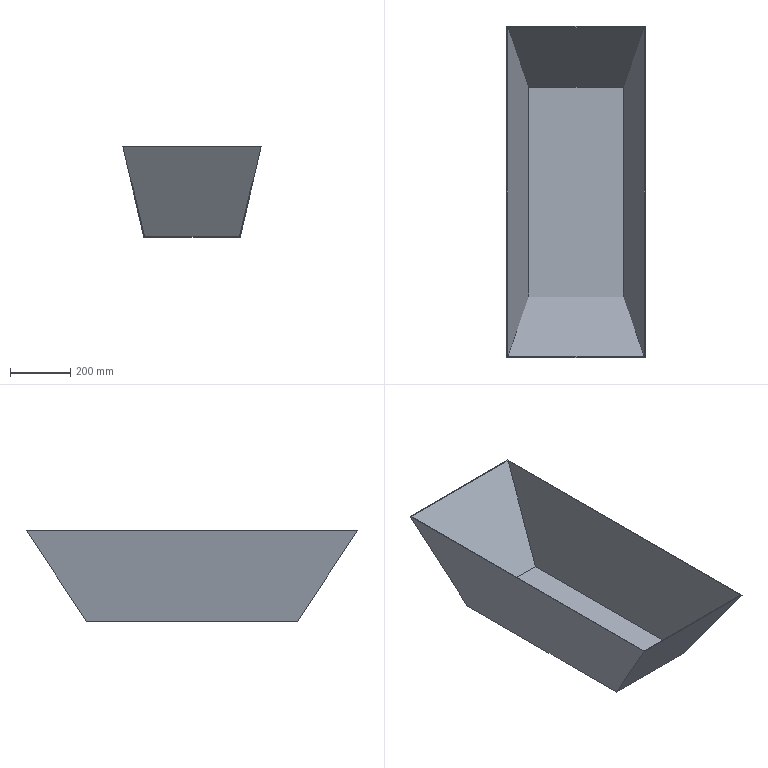Part | SolidWorks | features ICE 2, Extrusion 1, Shell 1 | 1 solid | 11 faces | box 460 x 1100 x 300 mm | volume 3149502 mm3 | plane 11
STEP:
#1=CARTESIAN_POINT('',(-160.,350.,-300.));
#2=VERTEX_POINT('',#1);
#3=CARTESIAN_POINT('',(160.,350.,-300.));
#4=VERTEX_POINT('',#3);
#5=CARTESIAN_POINT('',(-230.,350.,-300.));
#6=DIRECTION('',(1.,0.,0.));
#7=VECTOR('',#6,1000.);
#8=LINE('',#5,#7);
#9=EDGE_CURVE('',#2,#4,#8,.T.);
#10=ORIENTED_EDGE('',*,*,#9,.T.);
#11=CARTESIAN_POINT('',(160.,-350.,-300.));
#12=VERTEX_POINT('',#11);
#13=CARTESIAN_POINT('',(160.,-949.,-300.));
#14=DIRECTION('',(0.,1.,0.));
#15=VECTOR('',#14,1000.);
#16=LINE('',#13,#15);
#17=EDGE_CURVE('',#12,#4,#16,.T.);
#18=ORIENTED_EDGE('',*,*,#17,.F.);
#19=CARTESIAN_POINT('',(-160.,-350.,-300.));
#20=VERTEX_POINT('',#19);
#21=CARTESIAN_POINT('',(-230.,-350.,-300.));
#22=DIRECTION('',(1.,0.,0.));
#23=VECTOR('',#22,1000.);
#24=LINE('',#21,#23);
#25=EDGE_CURVE('',#20,#12,#24,.T.);
#26=ORIENTED_EDGE('',*,*,#25,.F.);
#27=CARTESIAN_POINT('',(-160.,-949.,-300.));
#28=DIRECTION('',(0.,1.,0.));
#29=VECTOR('',#28,1000.);
#30=LINE('',#27,#29);
#31=EDGE_CURVE('',#20,#2,#30,.T.);
#32=ORIENTED_EDGE('',*,*,#31,.T.);
#33=EDGE_LOOP('',(#10,#18,#26,#32));
#34=FACE_OUTER_BOUND('',#33,.T.);
#35=CARTESIAN_POINT('',(0.,0.,-300.));
#36=DIRECTION('',(0.,0.,1.));
#37=DIRECTION('',(1.,0.,0.));
#38=AXIS2_PLACEMENT_3D('',#35,#36,#37);
#39=PLANE('',#38);
#40=ADVANCED_FACE('',(#34),#39,.F.);
#41=CARTESIAN_POINT('',(226.919,-546.394,0.));
#42=VERTEX_POINT('',#41);
#43=CARTESIAN_POINT('',(226.919,546.394,0.));
#44=VERTEX_POINT('',#43);
#45=CARTESIAN_POINT('',(226.919,-949.,0.));
#46=DIRECTION('',(0.,1.,0.));
#47=VECTOR('',#46,1000.);
#48=LINE('',#45,#47);
#49=EDGE_CURVE('',#42,#44,#48,.T.);
#50=ORIENTED_EDGE('',*,*,#49,.F.);
#51=CARTESIAN_POINT('',(-226.919,-546.394,0.));
#52=VERTEX_POINT('',#51);
#53=CARTESIAN_POINT('',(-230.,-546.394,0.));
#54=DIRECTION('',(1.,0.,0.));
#55=VECTOR('',#54,1000.);
#56=LINE('',#53,#55);
#57=EDGE_CURVE('',#52,#42,#56,.T.);
#58=ORIENTED_EDGE('',*,*,#57,.F.);
#59=CARTESIAN_POINT('',(-226.919,546.394,0.));
#60=VERTEX_POINT('',#59);
#61=CARTESIAN_POINT('',(-226.919,-949.,0.));
#62=DIRECTION('',(0.,-1.,0.));
#63=VECTOR('',#62,1000.);
#64=LINE('',#61,#63);
#65=EDGE_CURVE('',#60,#52,#64,.T.);
#66=ORIENTED_EDGE('',*,*,#65,.F.);
#67=CARTESIAN_POINT('',(-230.,546.394,0.));
#68=DIRECTION('',(-1.,0.,0.));
#69=VECTOR('',#68,1000.);
#70=LINE('',#67,#69);
#71=EDGE_CURVE('',#44,#60,#70,.T.);
#72=ORIENTED_EDGE('',*,*,#71,.F.);
#73=EDGE_LOOP('',(#50,#58,#66,#72));
#74=FACE_BOUND('',#73,.T.);
#75=CARTESIAN_POINT('',(230.,-550.,0.));
#76=VERTEX_POINT('',#75);
#77=CARTESIAN_POINT('',(230.,550.,0.));
#78=VERTEX_POINT('',#77);
#79=CARTESIAN_POINT('',(230.,550.,0.));
#80=DIRECTION('',(0.,1.,0.));
#81=VECTOR('',#80,1000.);
#82=LINE('',#79,#81);
#83=EDGE_CURVE('',#76,#78,#82,.T.);
#84=ORIENTED_EDGE('',*,*,#83,.T.);
#85=CARTESIAN_POINT('',(-230.,550.,0.));
#86=VERTEX_POINT('',#85);
#87=CARTESIAN_POINT('',(-230.,550.,0.));
#88=DIRECTION('',(-1.,0.,0.));
#89=VECTOR('',#88,1000.);
#90=LINE('',#87,#89);
#91=EDGE_CURVE('',#78,#86,#90,.T.);
#92=ORIENTED_EDGE('',*,*,#91,.T.);
#93=CARTESIAN_POINT('',(-230.,-550.,0.));
#94=VERTEX_POINT('',#93);
#95=CARTESIAN_POINT('',(-230.,550.,0.));
#96=DIRECTION('',(0.,-1.,0.));
#97=VECTOR('',#96,1000.);
#98=LINE('',#95,#97);
#99=EDGE_CURVE('',#86,#94,#98,.T.);
#100=ORIENTED_EDGE('',*,*,#99,.T.);
#101=CARTESIAN_POINT('',(-230.,-550.,0.));
#102=DIRECTION('',(1.,0.,0.));
#103=VECTOR('',#102,1000.);
#104=LINE('',#101,#103);
#105=EDGE_CURVE('',#94,#76,#104,.T.);
#106=ORIENTED_EDGE('',*,*,#105,.T.);
#107=EDGE_LOOP('',(#84,#92,#100,#106));
#108=FACE_OUTER_BOUND('',#107,.T.);
#109=CARTESIAN_POINT('',(0.,0.,0.));
#110=DIRECTION('',(0.,0.,1.));
#111=DIRECTION('',(1.,0.,0.));
#112=AXIS2_PLACEMENT_3D('',#109,#110,#111);
#113=PLANE('',#112);
#114=ADVANCED_FACE('',(#74,#108),#113,.T.);
#115=ORIENTED_EDGE('',*,*,#91,.F.);
#116=CARTESIAN_POINT('',(213.291,502.261,-71.609));
#117=DIRECTION('',(-0.1906,-0.5445,-0.8168));
#118=VECTOR('',#117,1000.);
#119=LINE('',#116,#118);
#120=EDGE_CURVE('',#78,#4,#119,.T.);
#121=ORIENTED_EDGE('',*,*,#120,.T.);
#122=ORIENTED_EDGE('',*,*,#9,.F.);
#123=CARTESIAN_POINT('',(-230.,550.,0.));
#124=DIRECTION('',(-0.1906,0.5445,0.8168));
#125=VECTOR('',#124,1000.);
#126=LINE('',#123,#125);
#127=EDGE_CURVE('',#2,#86,#126,.T.);
#128=ORIENTED_EDGE('',*,*,#127,.T.);
#129=EDGE_LOOP('',(#115,#121,#122,#128));
#130=FACE_OUTER_BOUND('',#129,.T.);
#131=CARTESIAN_POINT('',(-230.,550.,0.));
#132=DIRECTION('',(0.,-0.8321,0.5547));
#133=DIRECTION('',(0.,-0.5547,-0.8321));
#134=AXIS2_PLACEMENT_3D('',#131,#132,#133);
#135=PLANE('',#134);
#136=ADVANCED_FACE('',(#130),#135,.F.);
#137=ORIENTED_EDGE('',*,*,#25,.T.);
#138=CARTESIAN_POINT('',(213.291,-502.261,-71.609));
#139=DIRECTION('',(0.1906,-0.5445,0.8168));
#140=VECTOR('',#139,1000.);
#141=LINE('',#138,#140);
#142=EDGE_CURVE('',#12,#76,#141,.T.);
#143=ORIENTED_EDGE('',*,*,#142,.T.);
#144=ORIENTED_EDGE('',*,*,#105,.F.);
#145=CARTESIAN_POINT('',(-230.,-550.,0.));
#146=DIRECTION('',(0.1906,0.5445,-0.8168));
#147=VECTOR('',#146,1000.);
#148=LINE('',#145,#147);
#149=EDGE_CURVE('',#94,#20,#148,.T.);
#150=ORIENTED_EDGE('',*,*,#149,.T.);
#151=EDGE_LOOP('',(#137,#143,#144,#150));
#152=FACE_OUTER_BOUND('',#151,.T.);
#153=CARTESIAN_POINT('',(-230.,-550.,0.));
#154=DIRECTION('',(0.,0.8321,0.5547));
#155=DIRECTION('',(0.,-0.5547,0.8321));
#156=AXIS2_PLACEMENT_3D('',#153,#154,#155);
#157=PLANE('',#156);
#158=ADVANCED_FACE('',(#152),#157,.F.);
#159=ORIENTED_EDGE('',*,*,#31,.F.);
#160=ORIENTED_EDGE('',*,*,#149,.F.);
#161=ORIENTED_EDGE('',*,*,#99,.F.);
#162=ORIENTED_EDGE('',*,*,#127,.F.);
#163=EDGE_LOOP('',(#159,#160,#161,#162));
#164=FACE_OUTER_BOUND('',#163,.T.);
#165=CARTESIAN_POINT('',(-230.,-949.,0.));
#166=DIRECTION('',(0.9738,0.,0.2272));
#167=DIRECTION('',(0.2272,0.,-0.9738));
#168=AXIS2_PLACEMENT_3D('',#165,#166,#167);
#169=PLANE('',#168);
#170=ADVANCED_FACE('',(#164),#169,.F.);
#171=ORIENTED_EDGE('',*,*,#83,.F.);
#172=ORIENTED_EDGE('',*,*,#142,.F.);
#173=ORIENTED_EDGE('',*,*,#17,.T.);
#174=ORIENTED_EDGE('',*,*,#120,.F.);
#175=EDGE_LOOP('',(#171,#172,#173,#174));
#176=FACE_OUTER_BOUND('',#175,.T.);
#177=CARTESIAN_POINT('',(230.,-949.,0.));
#178=DIRECTION('',(-0.9738,0.,0.2272));
#179=DIRECTION('',(0.2272,0.,0.9738));
#180=AXIS2_PLACEMENT_3D('',#177,#178,#179);
#181=PLANE('',#180);
#182=ADVANCED_FACE('',(#176),#181,.F.);
#183=CARTESIAN_POINT('',(-157.619,348.394,-297.));
#184=VERTEX_POINT('',#183);
#185=CARTESIAN_POINT('',(157.619,348.394,-297.));
#186=VERTEX_POINT('',#185);
#187=CARTESIAN_POINT('',(0.,348.394,-297.));
#188=DIRECTION('',(1.,0.,0.));
#189=VECTOR('',#188,1000.);
#190=LINE('',#187,#189);
#191=EDGE_CURVE('',#184,#186,#190,.T.);
#192=ORIENTED_EDGE('',*,*,#191,.F.);
#193=CARTESIAN_POINT('',(-157.619,-348.394,-297.));
#194=VERTEX_POINT('',#193);
#195=CARTESIAN_POINT('',(-157.619,0.,-297.));
#196=DIRECTION('',(0.,1.,0.));
#197=VECTOR('',#196,1000.);
#198=LINE('',#195,#197);
#199=EDGE_CURVE('',#194,#184,#198,.T.);
#200=ORIENTED_EDGE('',*,*,#199,.F.);
#201=CARTESIAN_POINT('',(157.619,-348.394,-297.));
#202=VERTEX_POINT('',#201);
#203=CARTESIAN_POINT('',(-230.,-348.394,-297.));
#204=DIRECTION('',(1.,0.,0.));
#205=VECTOR('',#204,1000.);
#206=LINE('',#203,#205);
#207=EDGE_CURVE('',#194,#202,#206,.T.);
#208=ORIENTED_EDGE('',*,*,#207,.T.);
#209=CARTESIAN_POINT('',(157.619,-949.,-297.));
#210=DIRECTION('',(0.,1.,0.));
#211=VECTOR('',#210,1000.);
#212=LINE('',#209,#211);
#213=EDGE_CURVE('',#202,#186,#212,.T.);
#214=ORIENTED_EDGE('',*,*,#213,.T.);
#215=EDGE_LOOP('',(#192,#200,#208,#214));
#216=FACE_OUTER_BOUND('',#215,.T.);
#217=CARTESIAN_POINT('',(0.,0.,-297.));
#218=DIRECTION('',(0.,0.,1.));
#219=DIRECTION('',(1.,0.,0.));
#220=AXIS2_PLACEMENT_3D('',#217,#218,#219);
#221=PLANE('',#220);
#222=ADVANCED_FACE('',(#216),#221,.T.);
#223=ORIENTED_EDGE('',*,*,#71,.T.);
#224=CARTESIAN_POINT('',(-227.405,547.783,2.083));
#225=DIRECTION('',(-0.1906,0.5445,0.8168));
#226=VECTOR('',#225,1000.);
#227=LINE('',#224,#226);
#228=EDGE_CURVE('',#184,#60,#227,.T.);
#229=ORIENTED_EDGE('',*,*,#228,.F.);
#230=ORIENTED_EDGE('',*,*,#191,.T.);
#231=CARTESIAN_POINT('',(210.697,500.044,-69.525));
#232=DIRECTION('',(-0.1906,-0.5445,-0.8168));
#233=VECTOR('',#232,1000.);
#234=LINE('',#231,#233);
#235=EDGE_CURVE('',#44,#186,#234,.T.);
#236=ORIENTED_EDGE('',*,*,#235,.F.);
#237=EDGE_LOOP('',(#223,#229,#230,#236));
#238=FACE_OUTER_BOUND('',#237,.T.);
#239=CARTESIAN_POINT('',(-230.,547.504,1.664));
#240=DIRECTION('',(0.,-0.8321,0.5547));
#241=DIRECTION('',(0.,-0.5547,-0.8321));
#242=AXIS2_PLACEMENT_3D('',#239,#240,#241);
#243=PLANE('',#242);
#244=ADVANCED_FACE('',(#238),#243,.T.);
#245=ORIENTED_EDGE('',*,*,#207,.F.);
#246=CARTESIAN_POINT('',(-227.405,-547.783,2.083));
#247=DIRECTION('',(0.1906,0.5445,-0.8168));
#248=VECTOR('',#247,1000.);
#249=LINE('',#246,#248);
#250=EDGE_CURVE('',#52,#194,#249,.T.);
#251=ORIENTED_EDGE('',*,*,#250,.F.);
#252=ORIENTED_EDGE('',*,*,#57,.T.);
#253=CARTESIAN_POINT('',(210.697,-500.044,-69.525));
#254=DIRECTION('',(0.1906,-0.5445,0.8168));
#255=VECTOR('',#254,1000.);
#256=LINE('',#253,#255);
#257=EDGE_CURVE('',#202,#42,#256,.T.);
#258=ORIENTED_EDGE('',*,*,#257,.F.);
#259=EDGE_LOOP('',(#245,#251,#252,#258));
#260=FACE_OUTER_BOUND('',#259,.T.);
#261=CARTESIAN_POINT('',(-230.,-547.504,1.664));
#262=DIRECTION('',(0.,0.8321,0.5547));
#263=DIRECTION('',(0.,-0.5547,0.8321));
#264=AXIS2_PLACEMENT_3D('',#261,#262,#263);
#265=PLANE('',#264);
#266=ADVANCED_FACE('',(#260),#265,.T.);
#267=ORIENTED_EDGE('',*,*,#199,.T.);
#268=ORIENTED_EDGE('',*,*,#228,.T.);
#269=ORIENTED_EDGE('',*,*,#65,.T.);
#270=ORIENTED_EDGE('',*,*,#250,.T.);
#271=EDGE_LOOP('',(#267,#268,#269,#270));
#272=FACE_OUTER_BOUND('',#271,.T.);
#273=CARTESIAN_POINT('',(-227.078,-949.,0.6817));
#274=DIRECTION('',(0.9738,0.,0.2272));
#275=DIRECTION('',(0.2272,0.,-0.9738));
#276=AXIS2_PLACEMENT_3D('',#273,#274,#275);
#277=PLANE('',#276);
#278=ADVANCED_FACE('',(#272),#277,.T.);
#279=ORIENTED_EDGE('',*,*,#49,.T.);
#280=ORIENTED_EDGE('',*,*,#235,.T.);
#281=ORIENTED_EDGE('',*,*,#213,.F.);
#282=ORIENTED_EDGE('',*,*,#257,.T.);
#283=EDGE_LOOP('',(#279,#280,#281,#282));
#284=FACE_OUTER_BOUND('',#283,.T.);
#285=CARTESIAN_POINT('',(227.078,-949.,0.6817));
#286=DIRECTION('',(-0.9738,0.,0.2272));
#287=DIRECTION('',(0.2272,0.,0.9738));
#288=AXIS2_PLACEMENT_3D('',#285,#286,#287);
#289=PLANE('',#288);
#290=ADVANCED_FACE('',(#284),#289,.T.);
#291=CLOSED_SHELL('',(#40,#114,#136,#158,#170,#182,#222,#244,#266,#278,#290));
#292=MANIFOLD_SOLID_BREP('',#291);
#293=CARTESIAN_POINT('',(0.,0.,0.));
#294=DIRECTION('',(0.,0.,1.));
#295=DIRECTION('',(1.,0.,0.));
#296=AXIS2_PLACEMENT_3D('',#293,#294,#295);
#297=(LENGTH_UNIT()NAMED_UNIT(*)SI_UNIT(.MILLI.,.METRE.));
#298=UNCERTAINTY_MEASURE_WITH_UNIT(LENGTH_MEASURE(0.00001),#297,'','');
#299=(NAMED_UNIT(*)PLANE_ANGLE_UNIT()SI_UNIT($,.RADIAN.));
#300=(NAMED_UNIT(*)SI_UNIT($,.STERADIAN.)SOLID_ANGLE_UNIT());
#301=(GEOMETRIC_REPRESENTATION_CONTEXT(3)GLOBAL_UNCERTAINTY_ASSIGNED_CONTEXT((#298))GLOBAL_UNIT_ASSIGNED_CONTEXT((#297,#299,#300))REPRESENTATION_CONTEXT('',''));
#302=ADVANCED_BREP_SHAPE_REPRESENTATION('',(#292,#296),#301);